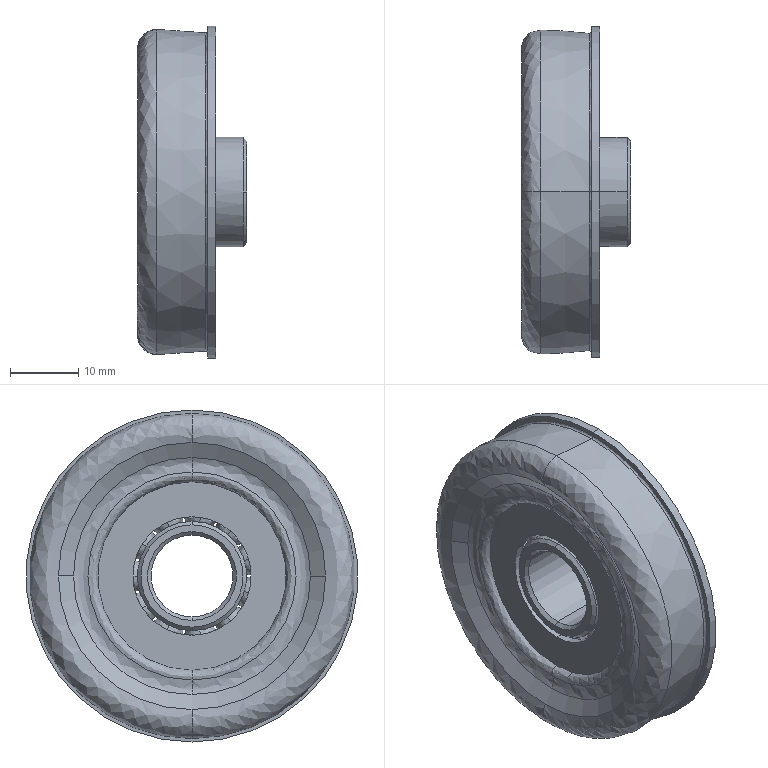Part | STEP file | 13 solids | 88 faces | box 15.973 x 48.6 x 48.6 mm | volume 7087 mm3 | spline 42 | cylinder 20 | cone 16 | plane 10 | commonest cylinder face diameters 16 x4 12 x2 17.363 x2 18.914 x2 22.858 x2 25.2 x2